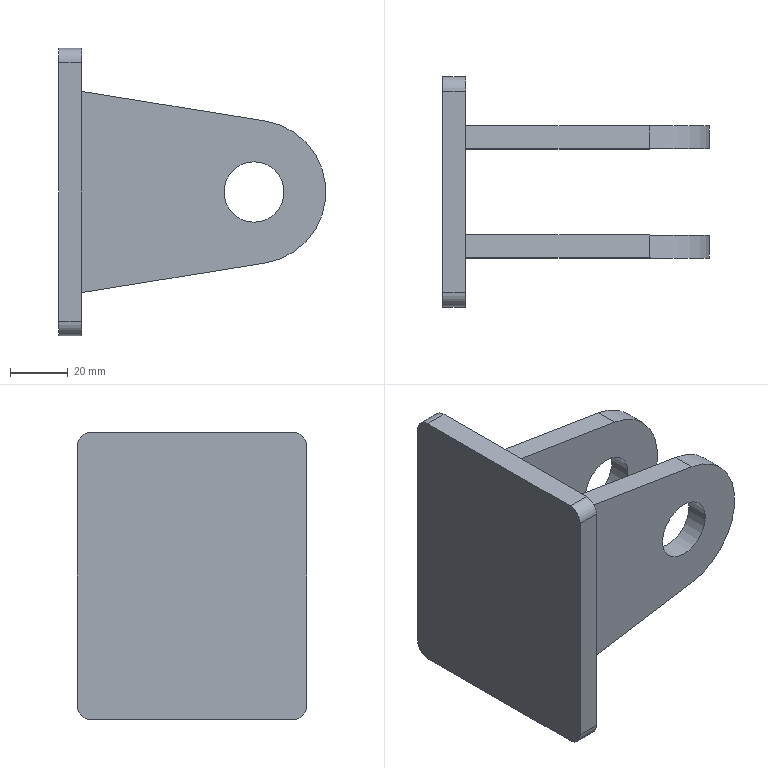Part | STEP file | HL4GZ-1.30.033 (cylinder mounting seat 1 weldment) | 3 solids | 24 faces | box 93 x 80 x 100 mm | volume 131918 mm3 | plane 16 | cylinder 8 | commonest cylinder face diameters 10 x4 21 x2 50 x2